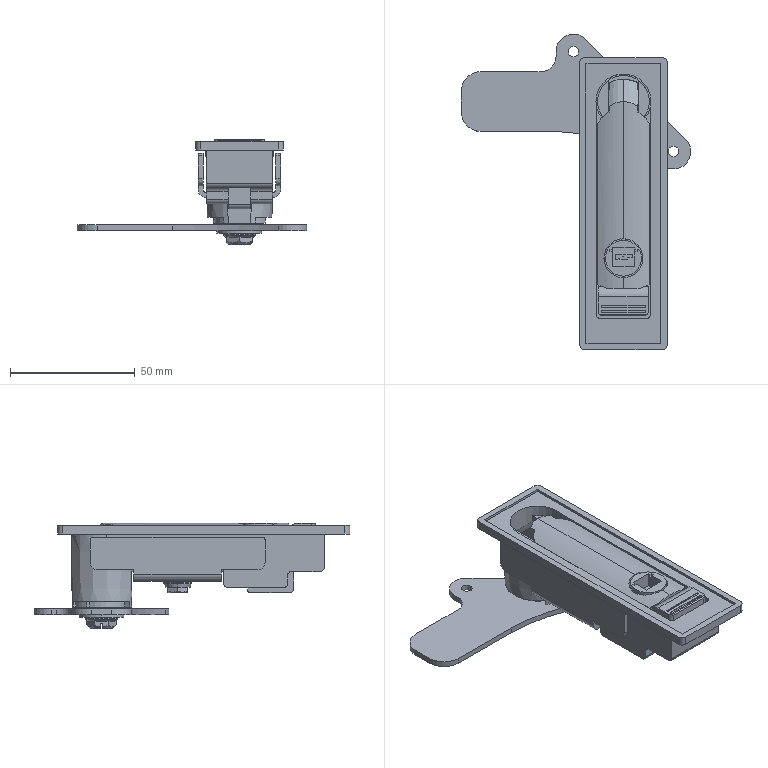Part | SolidWorks | features AEMSimFeature 1 | 3 solids | 369 faces | box 92 x 126.5 x 42.2 mm | volume 56869 mm3 | plane 225 | cylinder 107 | torus 19 | cone 18 | commonest cylinder face diameters 3.4 x9 6 x8 3 x7 0.8 x6 2 x6 1 x5